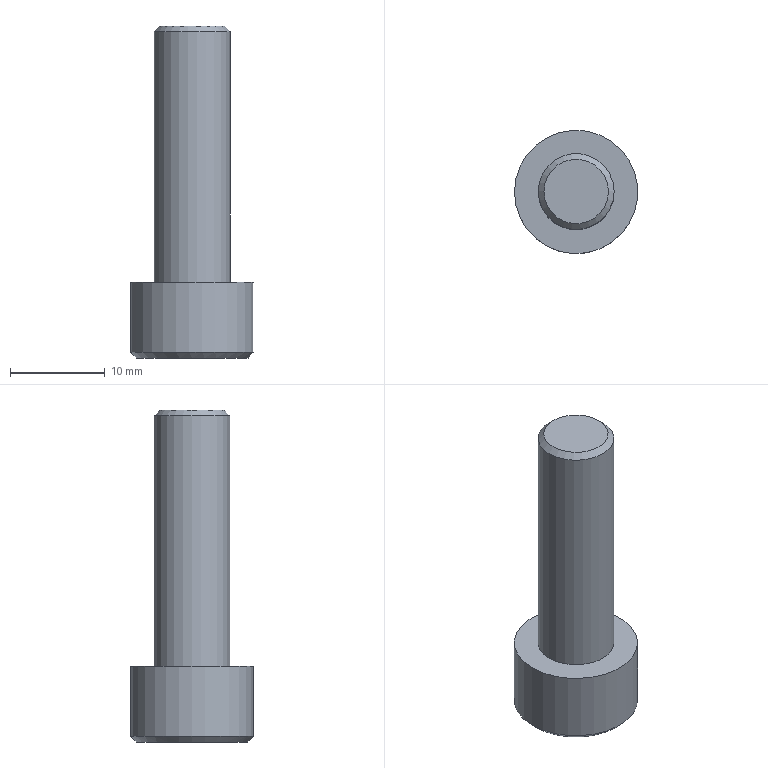Part | STEP file | M8.00-35.00 | 1 solid | 14 faces | box 13 x 13 x 35 mm | volume 2247 mm3 | plane 10 | cylinder 2 | cone 2 | commonest cylinder face diameters 8 x1 13 x1